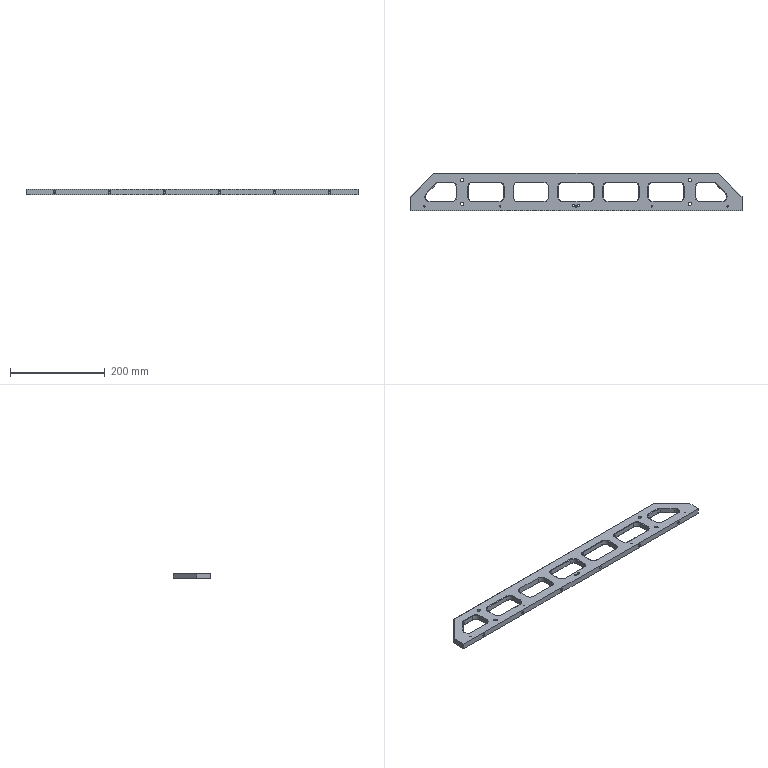Part | SolidWorks | features ICE 7, HoleWzd 4, Chamfer 1, Extrusion 1, Fillet 1 | 1 solid | 227 faces | box 700 x 80 x 12 mm | volume 406374 mm3 | plane 94 | cylinder 71 | cone 62 | commonest cylinder face diameters 20 x29 5 x16 3.3 x10 6.6 x8 11 x8